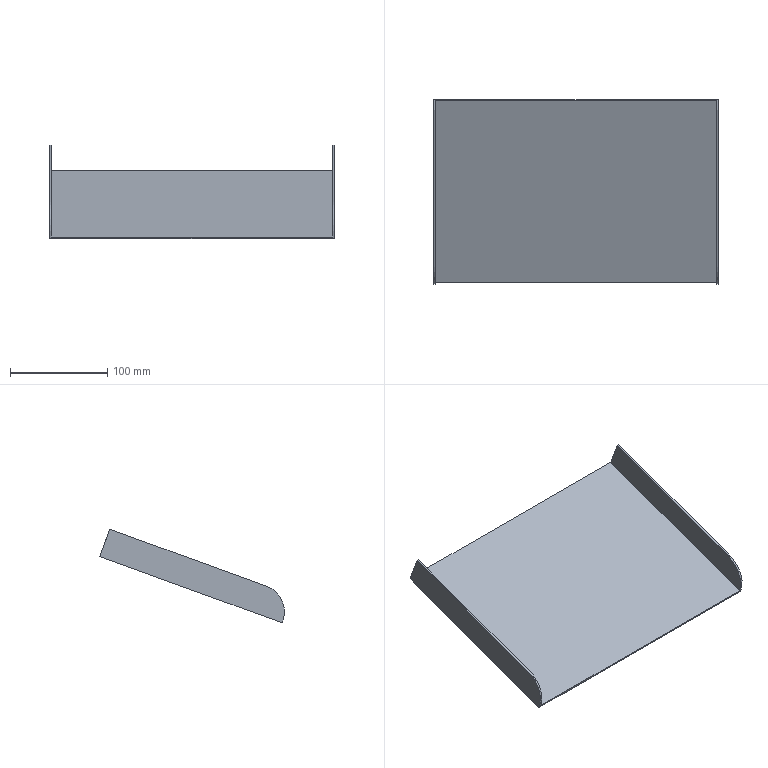Part | NX | features solid 2 | 1 solid | 12 faces | box 293.709 x 190.311 x 96.595 mm | volume 139211 mm3 | plane 10 | cylinder 2 | commonest cylinder face diameters 56 x2
STEP:
#1=CARTESIAN_POINT('',(372.,-997.939,-365.986));
#2=VERTEX_POINT('',#1);
#3=CARTESIAN_POINT('',(661.709,-997.939,-365.986));
#4=VERTEX_POINT('',#3);
#5=CARTESIAN_POINT('',(382.,-997.939,-365.986));
#6=DIRECTION('',(-1.,0.,0.));
#7=VECTOR('',#6,1000.);
#8=LINE('',#5,#7);
#9=EDGE_CURVE('',#2,#4,#8,.F.);
#10=ORIENTED_EDGE('',*,*,#9,.T.);
#11=CARTESIAN_POINT('',(661.709,-810.,-297.582));
#12=VERTEX_POINT('',#11);
#13=CARTESIAN_POINT('',(661.709,-838.191,-307.843));
#14=DIRECTION('',(0.,0.9397,0.342));
#15=VECTOR('',#14,1000.);
#16=LINE('',#13,#15);
#17=EDGE_CURVE('',#4,#12,#16,.T.);
#18=ORIENTED_EDGE('',*,*,#17,.T.);
#19=CARTESIAN_POINT('',(372.,-810.,-297.582));
#20=VERTEX_POINT('',#19);
#21=CARTESIAN_POINT('',(382.,-810.,-297.582));
#22=DIRECTION('',(1.,0.,0.));
#23=VECTOR('',#22,1000.);
#24=LINE('',#21,#23);
#25=EDGE_CURVE('',#20,#12,#24,.T.);
#26=ORIENTED_EDGE('',*,*,#25,.F.);
#27=CARTESIAN_POINT('',(372.,-838.191,-307.843));
#28=DIRECTION('',(0.,0.9397,0.342));
#29=VECTOR('',#28,1000.);
#30=LINE('',#27,#29);
#31=EDGE_CURVE('',#2,#20,#30,.T.);
#32=ORIENTED_EDGE('',*,*,#31,.F.);
#33=EDGE_LOOP('',(#10,#18,#26,#32));
#34=FACE_BOUND('',#33,.T.);
#35=CARTESIAN_POINT('',(382.,-838.191,-307.843));
#36=DIRECTION('',(0.,0.342,-0.9397));
#37=DIRECTION('',(-1.,0.,0.));
#38=AXIS2_PLACEMENT_3D('',#35,#36,#37);
#39=PLANE('',#38);
#40=ADVANCED_FACE('',(#34),#39,.F.);
#41=ORIENTED_EDGE('',*,*,#25,.T.);
#42=CARTESIAN_POINT('',(661.709,-819.577,-271.271));
#43=VERTEX_POINT('',#42);
#44=CARTESIAN_POINT('',(661.709,-809.316,-299.462));
#45=DIRECTION('',(0.,-0.342,0.9397));
#46=VECTOR('',#45,1000.);
#47=LINE('',#44,#46);
#48=EDGE_CURVE('',#12,#43,#47,.T.);
#49=ORIENTED_EDGE('',*,*,#48,.T.);
#50=CARTESIAN_POINT('',(663.709,-819.577,-271.271));
#51=VERTEX_POINT('',#50);
#52=CARTESIAN_POINT('',(663.709,-819.577,-271.271));
#53=DIRECTION('',(1.,0.,0.));
#54=VECTOR('',#53,1000.);
#55=LINE('',#52,#54);
#56=EDGE_CURVE('',#51,#43,#55,.F.);
#57=ORIENTED_EDGE('',*,*,#56,.F.);
#58=CARTESIAN_POINT('',(663.709,-809.316,-299.462));
#59=VERTEX_POINT('',#58);
#60=CARTESIAN_POINT('',(663.709,-809.316,-299.462));
#61=DIRECTION('',(0.,-0.342,0.9397));
#62=VECTOR('',#61,1000.);
#63=LINE('',#60,#62);
#64=EDGE_CURVE('',#59,#51,#63,.T.);
#65=ORIENTED_EDGE('',*,*,#64,.F.);
#66=CARTESIAN_POINT('',(370.,-809.316,-299.462));
#67=VERTEX_POINT('',#66);
#68=CARTESIAN_POINT('',(382.,-809.316,-299.462));
#69=DIRECTION('',(1.,0.,0.));
#70=VECTOR('',#69,1000.);
#71=LINE('',#68,#70);
#72=EDGE_CURVE('',#67,#59,#71,.T.);
#73=ORIENTED_EDGE('',*,*,#72,.F.);
#74=CARTESIAN_POINT('',(370.,-819.577,-271.271));
#75=VERTEX_POINT('',#74);
#76=CARTESIAN_POINT('',(370.,-809.316,-299.462));
#77=DIRECTION('',(0.,0.342,-0.9397));
#78=VECTOR('',#77,1000.);
#79=LINE('',#76,#78);
#80=EDGE_CURVE('',#67,#75,#79,.F.);
#81=ORIENTED_EDGE('',*,*,#80,.T.);
#82=CARTESIAN_POINT('',(372.,-819.577,-271.271));
#83=VERTEX_POINT('',#82);
#84=CARTESIAN_POINT('',(370.,-819.577,-271.271));
#85=DIRECTION('',(1.,0.,0.));
#86=VECTOR('',#85,1000.);
#87=LINE('',#84,#86);
#88=EDGE_CURVE('',#75,#83,#87,.T.);
#89=ORIENTED_EDGE('',*,*,#88,.T.);
#90=CARTESIAN_POINT('',(372.,-809.316,-299.462));
#91=DIRECTION('',(0.,-0.342,0.9397));
#92=VECTOR('',#91,1000.);
#93=LINE('',#90,#92);
#94=EDGE_CURVE('',#20,#83,#93,.T.);
#95=ORIENTED_EDGE('',*,*,#94,.F.);
#96=EDGE_LOOP('',(#41,#49,#57,#65,#73,#81,#89,#95));
#97=FACE_BOUND('',#96,.T.);
#98=CARTESIAN_POINT('',(382.,-809.316,-299.462));
#99=DIRECTION('',(0.,0.9397,0.342));
#100=DIRECTION('',(1.,0.,0.));
#101=AXIS2_PLACEMENT_3D('',#98,#99,#100);
#102=PLANE('',#101);
#103=ADVANCED_FACE('',(#97),#102,.T.);
#104=ORIENTED_EDGE('',*,*,#80,.F.);
#105=CARTESIAN_POINT('',(370.,-997.254,-367.866));
#106=VERTEX_POINT('',#105);
#107=CARTESIAN_POINT('',(370.,-837.507,-309.722));
#108=DIRECTION('',(0.,0.9397,0.342));
#109=VECTOR('',#108,1000.);
#110=LINE('',#107,#109);
#111=EDGE_CURVE('',#67,#106,#110,.F.);
#112=ORIENTED_EDGE('',*,*,#111,.T.);
#113=CARTESIAN_POINT('',(370.,-997.939,-365.986));
#114=VERTEX_POINT('',#113);
#115=CARTESIAN_POINT('',(370.,-997.254,-367.866));
#116=DIRECTION('',(0.,-0.342,0.9397));
#117=VECTOR('',#116,1000.);
#118=LINE('',#115,#117);
#119=EDGE_CURVE('',#106,#114,#118,.T.);
#120=ORIENTED_EDGE('',*,*,#119,.T.);
#121=CARTESIAN_POINT('',(370.,-981.204,-330.098));
#122=VERTEX_POINT('',#121);
#123=CARTESIAN_POINT('',(370.,-971.627,-356.41));
#124=DIRECTION('',(-1.,0.,0.));
#125=DIRECTION('',(0.,0.,1.));
#126=AXIS2_PLACEMENT_3D('',#123,#124,#125);
#127=CIRCLE('',#126,28.);
#128=EDGE_CURVE('',#114,#122,#127,.T.);
#129=ORIENTED_EDGE('',*,*,#128,.T.);
#130=CARTESIAN_POINT('',(370.,-819.577,-271.271));
#131=DIRECTION('',(0.,-0.9397,-0.342));
#132=VECTOR('',#131,1000.);
#133=LINE('',#130,#132);
#134=EDGE_CURVE('',#75,#122,#133,.T.);
#135=ORIENTED_EDGE('',*,*,#134,.F.);
#136=EDGE_LOOP('',(#104,#112,#120,#129,#135));
#137=FACE_BOUND('',#136,.T.);
#138=CARTESIAN_POINT('',(370.,-837.507,-309.722));
#139=DIRECTION('',(1.,0.,0.));
#140=DIRECTION('',(0.,-0.9397,-0.342));
#141=AXIS2_PLACEMENT_3D('',#138,#139,#140);
#142=PLANE('',#141);
#143=ADVANCED_FACE('',(#137),#142,.F.);
#144=CARTESIAN_POINT('',(663.709,-997.254,-367.866));
#145=VERTEX_POINT('',#144);
#146=CARTESIAN_POINT('',(382.,-997.254,-367.866));
#147=DIRECTION('',(1.,0.,0.));
#148=VECTOR('',#147,1000.);
#149=LINE('',#146,#148);
#150=EDGE_CURVE('',#106,#145,#149,.T.);
#151=ORIENTED_EDGE('',*,*,#150,.T.);
#152=CARTESIAN_POINT('',(663.709,-997.939,-365.986));
#153=VERTEX_POINT('',#152);
#154=CARTESIAN_POINT('',(663.709,-997.254,-367.866));
#155=DIRECTION('',(0.,0.342,-0.9397));
#156=VECTOR('',#155,1000.);
#157=LINE('',#154,#156);
#158=EDGE_CURVE('',#145,#153,#157,.F.);
#159=ORIENTED_EDGE('',*,*,#158,.T.);
#160=CARTESIAN_POINT('',(663.709,-997.939,-365.986));
#161=DIRECTION('',(-1.,0.,0.));
#162=VECTOR('',#161,1000.);
#163=LINE('',#160,#162);
#164=EDGE_CURVE('',#153,#4,#163,.T.);
#165=ORIENTED_EDGE('',*,*,#164,.T.);
#166=ORIENTED_EDGE('',*,*,#9,.F.);
#167=CARTESIAN_POINT('',(382.,-997.939,-365.986));
#168=DIRECTION('',(-1.,0.,0.));
#169=VECTOR('',#168,1000.);
#170=LINE('',#167,#169);
#171=EDGE_CURVE('',#114,#2,#170,.F.);
#172=ORIENTED_EDGE('',*,*,#171,.F.);
#173=ORIENTED_EDGE('',*,*,#119,.F.);
#174=EDGE_LOOP('',(#151,#159,#165,#166,#172,#173));
#175=FACE_BOUND('',#174,.T.);
#176=CARTESIAN_POINT('',(382.,-997.254,-367.866));
#177=DIRECTION('',(0.,0.9397,0.342));
#178=DIRECTION('',(1.,0.,0.));
#179=AXIS2_PLACEMENT_3D('',#176,#177,#178);
#180=PLANE('',#179);
#181=ADVANCED_FACE('',(#175),#180,.F.);
#182=CARTESIAN_POINT('',(663.709,-837.507,-309.722));
#183=DIRECTION('',(0.,-0.9397,-0.342));
#184=VECTOR('',#183,1000.);
#185=LINE('',#182,#184);
#186=EDGE_CURVE('',#59,#145,#185,.T.);
#187=ORIENTED_EDGE('',*,*,#186,.F.);
#188=ORIENTED_EDGE('',*,*,#64,.T.);
#189=CARTESIAN_POINT('',(663.709,-981.204,-330.098));
#190=VERTEX_POINT('',#189);
#191=CARTESIAN_POINT('',(663.709,-819.577,-271.271));
#192=DIRECTION('',(0.,-0.9397,-0.342));
#193=VECTOR('',#192,1000.);
#194=LINE('',#191,#193);
#195=EDGE_CURVE('',#51,#190,#194,.T.);
#196=ORIENTED_EDGE('',*,*,#195,.T.);
#197=CARTESIAN_POINT('',(663.709,-971.627,-356.41));
#198=DIRECTION('',(-1.,0.,0.));
#199=DIRECTION('',(0.,0.,1.));
#200=AXIS2_PLACEMENT_3D('',#197,#198,#199);
#201=CIRCLE('',#200,28.);
#202=EDGE_CURVE('',#190,#153,#201,.F.);
#203=ORIENTED_EDGE('',*,*,#202,.T.);
#204=ORIENTED_EDGE('',*,*,#158,.F.);
#205=EDGE_LOOP('',(#187,#188,#196,#203,#204));
#206=FACE_BOUND('',#205,.T.);
#207=CARTESIAN_POINT('',(663.709,-837.507,-309.722));
#208=DIRECTION('',(1.,0.,0.));
#209=DIRECTION('',(0.,-0.9397,-0.342));
#210=AXIS2_PLACEMENT_3D('',#207,#208,#209);
#211=PLANE('',#210);
#212=ADVANCED_FACE('',(#206),#211,.T.);
#213=ORIENTED_EDGE('',*,*,#72,.T.);
#214=ORIENTED_EDGE('',*,*,#186,.T.);
#215=ORIENTED_EDGE('',*,*,#150,.F.);
#216=ORIENTED_EDGE('',*,*,#111,.F.);
#217=EDGE_LOOP('',(#213,#214,#215,#216));
#218=FACE_BOUND('',#217,.T.);
#219=CARTESIAN_POINT('',(382.,-837.507,-309.722));
#220=DIRECTION('',(0.,0.342,-0.9397));
#221=DIRECTION('',(-1.,0.,0.));
#222=AXIS2_PLACEMENT_3D('',#219,#220,#221);
#223=PLANE('',#222);
#224=ADVANCED_FACE('',(#218),#223,.T.);
#225=CARTESIAN_POINT('',(372.,-981.204,-330.098));
#226=VERTEX_POINT('',#225);
#227=CARTESIAN_POINT('',(372.,-971.627,-356.41));
#228=DIRECTION('',(-1.,0.,0.));
#229=DIRECTION('',(0.,0.,1.));
#230=AXIS2_PLACEMENT_3D('',#227,#228,#229);
#231=CIRCLE('',#230,28.);
#232=EDGE_CURVE('',#226,#2,#231,.F.);
#233=ORIENTED_EDGE('',*,*,#232,.T.);
#234=ORIENTED_EDGE('',*,*,#31,.T.);
#235=ORIENTED_EDGE('',*,*,#94,.T.);
#236=CARTESIAN_POINT('',(372.,-819.577,-271.271));
#237=DIRECTION('',(0.,-0.9397,-0.342));
#238=VECTOR('',#237,1000.);
#239=LINE('',#236,#238);
#240=EDGE_CURVE('',#83,#226,#239,.T.);
#241=ORIENTED_EDGE('',*,*,#240,.T.);
#242=EDGE_LOOP('',(#233,#234,#235,#241));
#243=FACE_BOUND('',#242,.T.);
#244=CARTESIAN_POINT('',(372.,-809.316,-299.462));
#245=DIRECTION('',(-1.,0.,0.));
#246=DIRECTION('',(0.,0.,1.));
#247=AXIS2_PLACEMENT_3D('',#244,#245,#246);
#248=PLANE('',#247);
#249=ADVANCED_FACE('',(#243),#248,.F.);
#250=ORIENTED_EDGE('',*,*,#134,.T.);
#251=CARTESIAN_POINT('',(370.,-981.204,-330.098));
#252=DIRECTION('',(1.,0.,0.));
#253=VECTOR('',#252,1000.);
#254=LINE('',#251,#253);
#255=EDGE_CURVE('',#122,#226,#254,.T.);
#256=ORIENTED_EDGE('',*,*,#255,.T.);
#257=ORIENTED_EDGE('',*,*,#240,.F.);
#258=ORIENTED_EDGE('',*,*,#88,.F.);
#259=EDGE_LOOP('',(#250,#256,#257,#258));
#260=FACE_BOUND('',#259,.T.);
#261=CARTESIAN_POINT('',(370.,-819.577,-271.271));
#262=DIRECTION('',(0.,0.342,-0.9397));
#263=DIRECTION('',(0.,-0.9397,-0.342));
#264=AXIS2_PLACEMENT_3D('',#261,#262,#263);
#265=PLANE('',#264);
#266=ADVANCED_FACE('',(#260),#265,.F.);
#267=ORIENTED_EDGE('',*,*,#128,.F.);
#268=ORIENTED_EDGE('',*,*,#171,.T.);
#269=ORIENTED_EDGE('',*,*,#232,.F.);
#270=ORIENTED_EDGE('',*,*,#255,.F.);
#271=EDGE_LOOP('',(#267,#268,#269,#270));
#272=FACE_BOUND('',#271,.T.);
#273=CARTESIAN_POINT('',(370.,-971.627,-356.41));
#274=DIRECTION('',(-1.,0.,0.));
#275=DIRECTION('',(0.,0.,1.));
#276=AXIS2_PLACEMENT_3D('',#273,#274,#275);
#277=CYLINDRICAL_SURFACE('',#276,28.);
#278=ADVANCED_FACE('',(#272),#277,.T.);
#279=ORIENTED_EDGE('',*,*,#17,.F.);
#280=CARTESIAN_POINT('',(661.709,-981.204,-330.098));
#281=VERTEX_POINT('',#280);
#282=CARTESIAN_POINT('',(661.709,-971.627,-356.41));
#283=DIRECTION('',(-1.,0.,0.));
#284=DIRECTION('',(0.,0.,1.));
#285=AXIS2_PLACEMENT_3D('',#282,#283,#284);
#286=CIRCLE('',#285,28.);
#287=EDGE_CURVE('',#4,#281,#286,.T.);
#288=ORIENTED_EDGE('',*,*,#287,.T.);
#289=CARTESIAN_POINT('',(661.709,-819.577,-271.271));
#290=DIRECTION('',(0.,-0.9397,-0.342));
#291=VECTOR('',#290,1000.);
#292=LINE('',#289,#291);
#293=EDGE_CURVE('',#43,#281,#292,.T.);
#294=ORIENTED_EDGE('',*,*,#293,.F.);
#295=ORIENTED_EDGE('',*,*,#48,.F.);
#296=EDGE_LOOP('',(#279,#288,#294,#295));
#297=FACE_BOUND('',#296,.T.);
#298=CARTESIAN_POINT('',(661.709,-809.316,-299.462));
#299=DIRECTION('',(-1.,0.,0.));
#300=DIRECTION('',(0.,0.,1.));
#301=AXIS2_PLACEMENT_3D('',#298,#299,#300);
#302=PLANE('',#301);
#303=ADVANCED_FACE('',(#297),#302,.T.);
#304=ORIENTED_EDGE('',*,*,#293,.T.);
#305=CARTESIAN_POINT('',(663.709,-981.204,-330.098));
#306=DIRECTION('',(1.,0.,0.));
#307=VECTOR('',#306,1000.);
#308=LINE('',#305,#307);
#309=EDGE_CURVE('',#281,#190,#308,.T.);
#310=ORIENTED_EDGE('',*,*,#309,.T.);
#311=ORIENTED_EDGE('',*,*,#195,.F.);
#312=ORIENTED_EDGE('',*,*,#56,.T.);
#313=EDGE_LOOP('',(#304,#310,#311,#312));
#314=FACE_BOUND('',#313,.T.);
#315=CARTESIAN_POINT('',(663.709,-819.577,-271.271));
#316=DIRECTION('',(0.,0.342,-0.9397));
#317=DIRECTION('',(0.,-0.9397,-0.342));
#318=AXIS2_PLACEMENT_3D('',#315,#316,#317);
#319=PLANE('',#318);
#320=ADVANCED_FACE('',(#314),#319,.F.);
#321=ORIENTED_EDGE('',*,*,#202,.F.);
#322=ORIENTED_EDGE('',*,*,#309,.F.);
#323=ORIENTED_EDGE('',*,*,#287,.F.);
#324=ORIENTED_EDGE('',*,*,#164,.F.);
#325=EDGE_LOOP('',(#321,#322,#323,#324));
#326=FACE_BOUND('',#325,.T.);
#327=CARTESIAN_POINT('',(663.709,-971.627,-356.41));
#328=DIRECTION('',(1.,0.,0.));
#329=DIRECTION('',(0.,0.,-1.));
#330=AXIS2_PLACEMENT_3D('',#327,#328,#329);
#331=CYLINDRICAL_SURFACE('',#330,28.);
#332=ADVANCED_FACE('',(#326),#331,.T.);
#333=CLOSED_SHELL('',(#40,#103,#143,#181,#212,#224,#249,#266,#278,#303,#320,#332));
#334=MANIFOLD_SOLID_BREP('',#333);
#335=(LENGTH_UNIT()NAMED_UNIT(*)SI_UNIT(.MILLI.,.METRE.));
#336=UNCERTAINTY_MEASURE_WITH_UNIT(LENGTH_MEASURE(0.00001),#335,'','');
#337=(NAMED_UNIT(*)PLANE_ANGLE_UNIT()SI_UNIT($,.RADIAN.));
#338=(NAMED_UNIT(*)SI_UNIT($,.STERADIAN.)SOLID_ANGLE_UNIT());
#339=(GEOMETRIC_REPRESENTATION_CONTEXT(3)GLOBAL_UNCERTAINTY_ASSIGNED_CONTEXT((#336))GLOBAL_UNIT_ASSIGNED_CONTEXT((#335,#337,#338))REPRESENTATION_CONTEXT('',''));
#340=ADVANCED_BREP_SHAPE_REPRESENTATION('',(#334),#339);